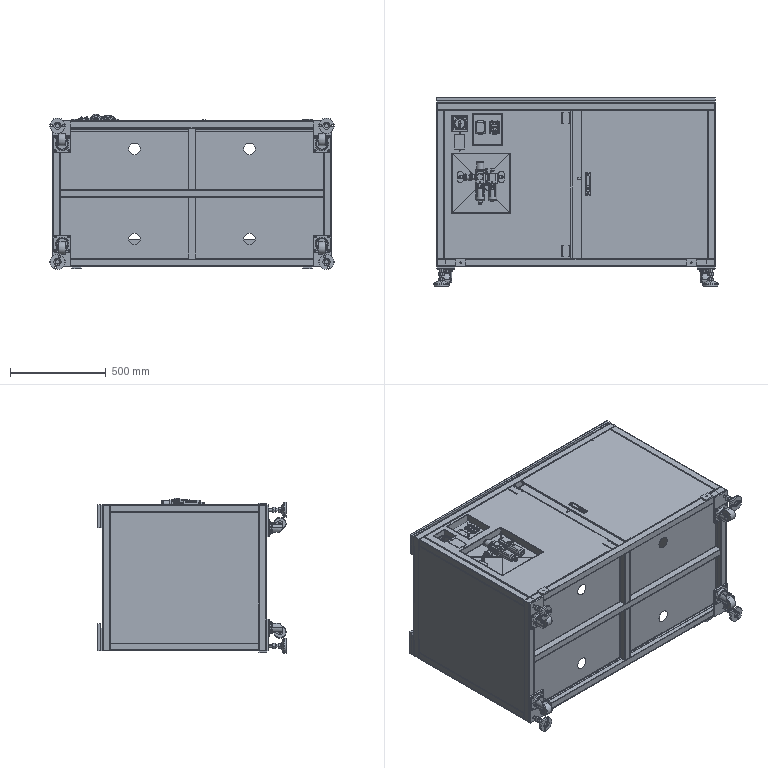Part | SolidWorks | features ReferencePattern 4, CompositeCurve 1, MirrorCompFeat 1 | 129 solids | 7157 faces | volume 37015208 mm3 | plane 3797 | cylinder 2088 | spline 728 | cone 312 | torus 186 | sphere 46 | commonest cylinder face diameters 1 x375 4 x230 2 x191 6.8 x124 0.6 x79 3 x65